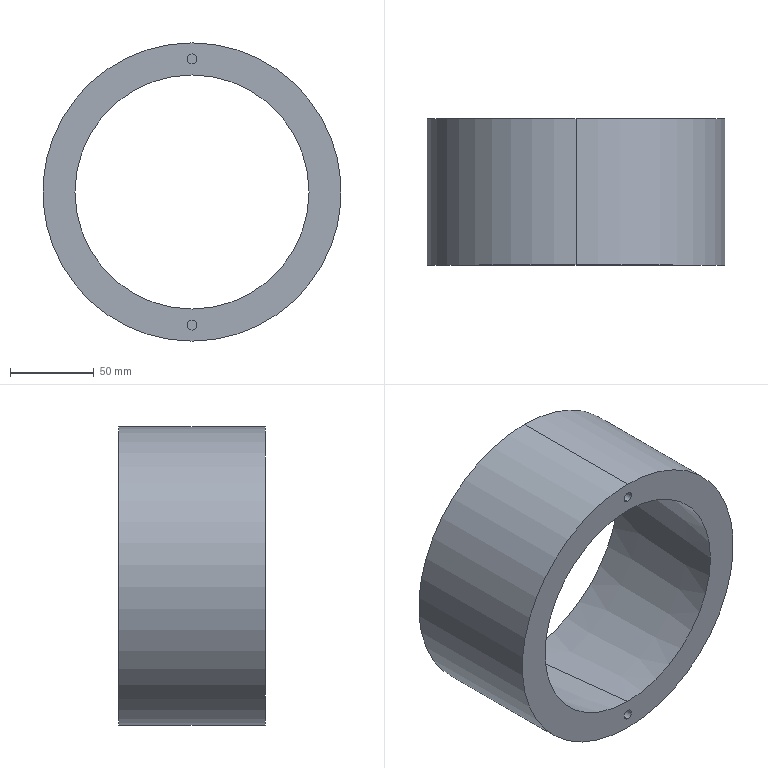Part | STEP file | waitao | 1 solid | 12 faces | box 178.3 x 87.518 x 178.3 mm | volume 654591 mm3 | cylinder 6 | plane 4 | cone 2 | commonest cylinder face diameters 6 x4 178.3 x2
STEP:
#1=CARTESIAN_POINT('',(0.,-167.046,82.551));
#2=VERTEX_POINT('',#1);
#3=CARTESIAN_POINT('',(0.,-167.046,76.551));
#4=VERTEX_POINT('',#3);
#5=CARTESIAN_POINT('',(0.,-167.046,79.551));
#6=DIRECTION('',(0.,-1.,0.));
#7=DIRECTION('',(0.,0.,-1.));
#8=AXIS2_PLACEMENT_3D('',#5,#6,#7);
#9=CIRCLE('',#8,3.);
#10=EDGE_CURVE('',#2,#4,#9,.T.);
#11=ORIENTED_EDGE('',*,*,#10,.F.);
#12=CARTESIAN_POINT('',(0.,-177.046,82.551));
#13=VERTEX_POINT('',#12);
#14=CARTESIAN_POINT('',(0.,-167.046,82.551));
#15=DIRECTION('',(0.,-1.,0.));
#16=VECTOR('',#15,1000.);
#17=LINE('',#14,#16);
#18=EDGE_CURVE('',#2,#13,#17,.T.);
#19=ORIENTED_EDGE('',*,*,#18,.T.);
#20=CARTESIAN_POINT('',(0.,-177.046,76.551));
#21=VERTEX_POINT('',#20);
#22=CARTESIAN_POINT('',(0.,-177.046,79.551));
#23=DIRECTION('',(0.,-1.,0.));
#24=DIRECTION('',(0.,0.,-1.));
#25=AXIS2_PLACEMENT_3D('',#22,#23,#24);
#26=CIRCLE('',#25,3.);
#27=EDGE_CURVE('',#13,#21,#26,.T.);
#28=ORIENTED_EDGE('',*,*,#27,.T.);
#29=CARTESIAN_POINT('',(0.,-167.046,76.551));
#30=DIRECTION('',(0.,-1.,0.));
#31=VECTOR('',#30,1000.);
#32=LINE('',#29,#31);
#33=EDGE_CURVE('',#4,#21,#32,.T.);
#34=ORIENTED_EDGE('',*,*,#33,.F.);
#35=EDGE_LOOP('',(#11,#19,#28,#34));
#36=FACE_OUTER_BOUND('',#35,.T.);
#37=CARTESIAN_POINT('',(0.,-167.046,79.551));
#38=DIRECTION('',(0.,-1.,0.));
#39=DIRECTION('',(0.,0.,-1.));
#40=AXIS2_PLACEMENT_3D('',#37,#38,#39);
#41=CYLINDRICAL_SURFACE('',#40,3.);
#42=ADVANCED_FACE('',(#36),#41,.F.);
#43=CARTESIAN_POINT('',(0.,-167.046,-76.551));
#44=VERTEX_POINT('',#43);
#45=CARTESIAN_POINT('',(0.,-167.046,-82.551));
#46=VERTEX_POINT('',#45);
#47=CARTESIAN_POINT('',(0.,-167.046,-79.551));
#48=DIRECTION('',(0.,-1.,0.));
#49=DIRECTION('',(0.,0.,-1.));
#50=AXIS2_PLACEMENT_3D('',#47,#48,#49);
#51=CIRCLE('',#50,3.);
#52=EDGE_CURVE('',#44,#46,#51,.T.);
#53=ORIENTED_EDGE('',*,*,#52,.F.);
#54=CARTESIAN_POINT('',(0.,-177.046,-76.551));
#55=VERTEX_POINT('',#54);
#56=CARTESIAN_POINT('',(0.,-167.046,-76.551));
#57=DIRECTION('',(0.,-1.,0.));
#58=VECTOR('',#57,1000.);
#59=LINE('',#56,#58);
#60=EDGE_CURVE('',#44,#55,#59,.T.);
#61=ORIENTED_EDGE('',*,*,#60,.T.);
#62=CARTESIAN_POINT('',(0.,-177.046,-82.551));
#63=VERTEX_POINT('',#62);
#64=CARTESIAN_POINT('',(0.,-177.046,-79.551));
#65=DIRECTION('',(0.,-1.,0.));
#66=DIRECTION('',(0.,0.,-1.));
#67=AXIS2_PLACEMENT_3D('',#64,#65,#66);
#68=CIRCLE('',#67,3.);
#69=EDGE_CURVE('',#55,#63,#68,.T.);
#70=ORIENTED_EDGE('',*,*,#69,.T.);
#71=CARTESIAN_POINT('',(0.,-167.046,-82.551));
#72=DIRECTION('',(0.,-1.,0.));
#73=VECTOR('',#72,1000.);
#74=LINE('',#71,#73);
#75=EDGE_CURVE('',#46,#63,#74,.T.);
#76=ORIENTED_EDGE('',*,*,#75,.F.);
#77=EDGE_LOOP('',(#53,#61,#70,#76));
#78=FACE_OUTER_BOUND('',#77,.T.);
#79=CARTESIAN_POINT('',(0.,-167.046,-79.551));
#80=DIRECTION('',(0.,-1.,0.));
#81=DIRECTION('',(0.,0.,-1.));
#82=AXIS2_PLACEMENT_3D('',#79,#80,#81);
#83=CYLINDRICAL_SURFACE('',#82,3.);
#84=ADVANCED_FACE('',(#78),#83,.F.);
#85=CARTESIAN_POINT('',(0.,-177.046,-69.951));
#86=VERTEX_POINT('',#85);
#87=CARTESIAN_POINT('',(0.,-177.046,69.951));
#88=VERTEX_POINT('',#87);
#89=CARTESIAN_POINT('',(0.,-177.046,0.));
#90=DIRECTION('',(0.,1.,0.));
#91=DIRECTION('',(0.,0.,1.));
#92=AXIS2_PLACEMENT_3D('',#89,#90,#91);
#93=CIRCLE('',#92,69.951);
#94=EDGE_CURVE('',#86,#88,#93,.T.);
#95=ORIENTED_EDGE('',*,*,#94,.F.);
#96=CARTESIAN_POINT('',(0.,-89.528,-79.15));
#97=VERTEX_POINT('',#96);
#98=CARTESIAN_POINT('',(0.,-89.528,-79.15));
#99=DIRECTION('',(0.,0.9945,-0.1045));
#100=VECTOR('',#99,1000.);
#101=LINE('',#98,#100);
#102=EDGE_CURVE('',#86,#97,#101,.T.);
#103=ORIENTED_EDGE('',*,*,#102,.T.);
#104=CARTESIAN_POINT('',(0.,-89.528,79.15));
#105=VERTEX_POINT('',#104);
#106=CARTESIAN_POINT('',(0.,-89.528,0.));
#107=DIRECTION('',(0.,1.,0.));
#108=DIRECTION('',(0.,0.,1.));
#109=AXIS2_PLACEMENT_3D('',#106,#107,#108);
#110=CIRCLE('',#109,79.15);
#111=EDGE_CURVE('',#97,#105,#110,.T.);
#112=ORIENTED_EDGE('',*,*,#111,.T.);
#113=CARTESIAN_POINT('',(0.,-89.528,79.15));
#114=DIRECTION('',(0.,0.9945,0.1045));
#115=VECTOR('',#114,1000.);
#116=LINE('',#113,#115);
#117=EDGE_CURVE('',#88,#105,#116,.T.);
#118=ORIENTED_EDGE('',*,*,#117,.F.);
#119=EDGE_LOOP('',(#95,#103,#112,#118));
#120=FACE_OUTER_BOUND('',#119,.T.);
#121=CARTESIAN_POINT('',(0.,-89.528,0.));
#122=DIRECTION('',(0.,1.,0.));
#123=DIRECTION('',(0.,0.,1.));
#124=AXIS2_PLACEMENT_3D('',#121,#122,#123);
#125=CONICAL_SURFACE('',#124,79.15,0.1047);
#126=ADVANCED_FACE('',(#120),#125,.F.);
#127=CARTESIAN_POINT('',(0.,-177.046,89.15));
#128=VERTEX_POINT('',#127);
#129=CARTESIAN_POINT('',(0.,-177.046,-89.15));
#130=VERTEX_POINT('',#129);
#131=CARTESIAN_POINT('',(0.,-177.046,0.));
#132=DIRECTION('',(0.,1.,0.));
#133=DIRECTION('',(0.,0.,1.));
#134=AXIS2_PLACEMENT_3D('',#131,#132,#133);
#135=CIRCLE('',#134,89.15);
#136=EDGE_CURVE('',#128,#130,#135,.T.);
#137=ORIENTED_EDGE('',*,*,#136,.T.);
#138=CARTESIAN_POINT('',(0.,-89.528,-89.15));
#139=VERTEX_POINT('',#138);
#140=CARTESIAN_POINT('',(0.,0.,-89.15));
#141=DIRECTION('',(0.,1.,0.));
#142=VECTOR('',#141,1000.);
#143=LINE('',#140,#142);
#144=EDGE_CURVE('',#130,#139,#143,.T.);
#145=ORIENTED_EDGE('',*,*,#144,.T.);
#146=CARTESIAN_POINT('',(0.,-89.528,89.15));
#147=VERTEX_POINT('',#146);
#148=CARTESIAN_POINT('',(0.,-89.528,0.));
#149=DIRECTION('',(0.,1.,0.));
#150=DIRECTION('',(0.,0.,1.));
#151=AXIS2_PLACEMENT_3D('',#148,#149,#150);
#152=CIRCLE('',#151,89.15);
#153=EDGE_CURVE('',#147,#139,#152,.T.);
#154=ORIENTED_EDGE('',*,*,#153,.F.);
#155=CARTESIAN_POINT('',(0.,0.,89.15));
#156=DIRECTION('',(0.,1.,0.));
#157=VECTOR('',#156,1000.);
#158=LINE('',#155,#157);
#159=EDGE_CURVE('',#128,#147,#158,.T.);
#160=ORIENTED_EDGE('',*,*,#159,.F.);
#161=EDGE_LOOP('',(#137,#145,#154,#160));
#162=FACE_OUTER_BOUND('',#161,.T.);
#163=CARTESIAN_POINT('',(0.,0.,0.));
#164=DIRECTION('',(0.,1.,0.));
#165=DIRECTION('',(0.,0.,1.));
#166=AXIS2_PLACEMENT_3D('',#163,#164,#165);
#167=CYLINDRICAL_SURFACE('',#166,89.15);
#168=ADVANCED_FACE('',(#162),#167,.T.);
#169=CARTESIAN_POINT('',(0.,-89.528,0.));
#170=DIRECTION('',(0.,1.,0.));
#171=DIRECTION('',(0.,0.,1.));
#172=AXIS2_PLACEMENT_3D('',#169,#170,#171);
#173=CIRCLE('',#172,79.15);
#174=EDGE_CURVE('',#105,#97,#173,.T.);
#175=ORIENTED_EDGE('',*,*,#174,.F.);
#176=ORIENTED_EDGE('',*,*,#111,.F.);
#177=EDGE_LOOP('',(#175,#176));
#178=FACE_BOUND('',#177,.T.);
#179=ORIENTED_EDGE('',*,*,#153,.T.);
#180=CARTESIAN_POINT('',(0.,-89.528,0.));
#181=DIRECTION('',(0.,1.,0.));
#182=DIRECTION('',(0.,0.,1.));
#183=AXIS2_PLACEMENT_3D('',#180,#181,#182);
#184=CIRCLE('',#183,89.15);
#185=EDGE_CURVE('',#139,#147,#184,.T.);
#186=ORIENTED_EDGE('',*,*,#185,.T.);
#187=EDGE_LOOP('',(#179,#186));
#188=FACE_OUTER_BOUND('',#187,.T.);
#189=CARTESIAN_POINT('',(79.15,-89.528,0.));
#190=DIRECTION('',(0.,-1.,0.));
#191=DIRECTION('',(0.,0.,-1.));
#192=AXIS2_PLACEMENT_3D('',#189,#190,#191);
#193=PLANE('',#192);
#194=ADVANCED_FACE('',(#178,#188),#193,.F.);
#195=ORIENTED_EDGE('',*,*,#144,.F.);
#196=CARTESIAN_POINT('',(0.,-177.046,0.));
#197=DIRECTION('',(0.,1.,0.));
#198=DIRECTION('',(0.,0.,1.));
#199=AXIS2_PLACEMENT_3D('',#196,#197,#198);
#200=CIRCLE('',#199,89.15);
#201=EDGE_CURVE('',#130,#128,#200,.T.);
#202=ORIENTED_EDGE('',*,*,#201,.T.);
#203=ORIENTED_EDGE('',*,*,#159,.T.);
#204=ORIENTED_EDGE('',*,*,#185,.F.);
#205=EDGE_LOOP('',(#195,#202,#203,#204));
#206=FACE_OUTER_BOUND('',#205,.T.);
#207=CARTESIAN_POINT('',(0.,0.,0.));
#208=DIRECTION('',(0.,1.,0.));
#209=DIRECTION('',(0.,0.,1.));
#210=AXIS2_PLACEMENT_3D('',#207,#208,#209);
#211=CYLINDRICAL_SURFACE('',#210,89.15);
#212=ADVANCED_FACE('',(#206),#211,.T.);
#213=CARTESIAN_POINT('',(0.,-177.046,79.551));
#214=DIRECTION('',(0.,-1.,0.));
#215=DIRECTION('',(0.,0.,-1.));
#216=AXIS2_PLACEMENT_3D('',#213,#214,#215);
#217=CIRCLE('',#216,3.);
#218=EDGE_CURVE('',#21,#13,#217,.T.);
#219=ORIENTED_EDGE('',*,*,#218,.F.);
#220=ORIENTED_EDGE('',*,*,#27,.F.);
#221=EDGE_LOOP('',(#219,#220));
#222=FACE_BOUND('',#221,.T.);
#223=CARTESIAN_POINT('',(0.,-177.046,-79.551));
#224=DIRECTION('',(0.,-1.,0.));
#225=DIRECTION('',(0.,0.,-1.));
#226=AXIS2_PLACEMENT_3D('',#223,#224,#225);
#227=CIRCLE('',#226,3.);
#228=EDGE_CURVE('',#63,#55,#227,.T.);
#229=ORIENTED_EDGE('',*,*,#228,.F.);
#230=ORIENTED_EDGE('',*,*,#69,.F.);
#231=EDGE_LOOP('',(#229,#230));
#232=FACE_BOUND('',#231,.T.);
#233=ORIENTED_EDGE('',*,*,#136,.F.);
#234=ORIENTED_EDGE('',*,*,#201,.F.);
#235=EDGE_LOOP('',(#233,#234));
#236=FACE_OUTER_BOUND('',#235,.T.);
#237=CARTESIAN_POINT('',(0.,-177.046,0.));
#238=DIRECTION('',(0.,1.,0.));
#239=DIRECTION('',(0.,0.,1.));
#240=AXIS2_PLACEMENT_3D('',#237,#238,#239);
#241=CIRCLE('',#240,69.951);
#242=EDGE_CURVE('',#88,#86,#241,.T.);
#243=ORIENTED_EDGE('',*,*,#242,.T.);
#244=ORIENTED_EDGE('',*,*,#94,.T.);
#245=EDGE_LOOP('',(#243,#244));
#246=FACE_BOUND('',#245,.T.);
#247=CARTESIAN_POINT('',(89.15,-177.046,0.));
#248=DIRECTION('',(0.,1.,0.));
#249=DIRECTION('',(0.,0.,1.));
#250=AXIS2_PLACEMENT_3D('',#247,#248,#249);
#251=PLANE('',#250);
#252=ADVANCED_FACE('',(#222,#232,#236,#246),#251,.F.);
#253=ORIENTED_EDGE('',*,*,#102,.F.);
#254=ORIENTED_EDGE('',*,*,#242,.F.);
#255=ORIENTED_EDGE('',*,*,#117,.T.);
#256=ORIENTED_EDGE('',*,*,#174,.T.);
#257=EDGE_LOOP('',(#253,#254,#255,#256));
#258=FACE_OUTER_BOUND('',#257,.T.);
#259=CARTESIAN_POINT('',(0.,-89.528,0.));
#260=DIRECTION('',(0.,1.,0.));
#261=DIRECTION('',(0.,0.,1.));
#262=AXIS2_PLACEMENT_3D('',#259,#260,#261);
#263=CONICAL_SURFACE('',#262,79.15,0.1047);
#264=ADVANCED_FACE('',(#258),#263,.F.);
#265=ORIENTED_EDGE('',*,*,#60,.F.);
#266=CARTESIAN_POINT('',(0.,-167.046,-79.551));
#267=DIRECTION('',(0.,-1.,0.));
#268=DIRECTION('',(0.,0.,-1.));
#269=AXIS2_PLACEMENT_3D('',#266,#267,#268);
#270=CIRCLE('',#269,3.);
#271=EDGE_CURVE('',#46,#44,#270,.T.);
#272=ORIENTED_EDGE('',*,*,#271,.F.);
#273=ORIENTED_EDGE('',*,*,#75,.T.);
#274=ORIENTED_EDGE('',*,*,#228,.T.);
#275=EDGE_LOOP('',(#265,#272,#273,#274));
#276=FACE_OUTER_BOUND('',#275,.T.);
#277=CARTESIAN_POINT('',(0.,-167.046,-79.551));
#278=DIRECTION('',(0.,-1.,0.));
#279=DIRECTION('',(0.,0.,-1.));
#280=AXIS2_PLACEMENT_3D('',#277,#278,#279);
#281=CYLINDRICAL_SURFACE('',#280,3.);
#282=ADVANCED_FACE('',(#276),#281,.F.);
#283=ORIENTED_EDGE('',*,*,#271,.T.);
#284=ORIENTED_EDGE('',*,*,#52,.T.);
#285=EDGE_LOOP('',(#283,#284));
#286=FACE_OUTER_BOUND('',#285,.T.);
#287=CARTESIAN_POINT('',(0.,-167.046,-79.551));
#288=DIRECTION('',(0.,-1.,0.));
#289=DIRECTION('',(0.,0.,-1.));
#290=AXIS2_PLACEMENT_3D('',#287,#288,#289);
#291=PLANE('',#290);
#292=ADVANCED_FACE('',(#286),#291,.T.);
#293=ORIENTED_EDGE('',*,*,#18,.F.);
#294=CARTESIAN_POINT('',(0.,-167.046,79.551));
#295=DIRECTION('',(0.,-1.,0.));
#296=DIRECTION('',(0.,0.,-1.));
#297=AXIS2_PLACEMENT_3D('',#294,#295,#296);
#298=CIRCLE('',#297,3.);
#299=EDGE_CURVE('',#4,#2,#298,.T.);
#300=ORIENTED_EDGE('',*,*,#299,.F.);
#301=ORIENTED_EDGE('',*,*,#33,.T.);
#302=ORIENTED_EDGE('',*,*,#218,.T.);
#303=EDGE_LOOP('',(#293,#300,#301,#302));
#304=FACE_OUTER_BOUND('',#303,.T.);
#305=CARTESIAN_POINT('',(0.,-167.046,79.551));
#306=DIRECTION('',(0.,-1.,0.));
#307=DIRECTION('',(0.,0.,-1.));
#308=AXIS2_PLACEMENT_3D('',#305,#306,#307);
#309=CYLINDRICAL_SURFACE('',#308,3.);
#310=ADVANCED_FACE('',(#304),#309,.F.);
#311=ORIENTED_EDGE('',*,*,#299,.T.);
#312=ORIENTED_EDGE('',*,*,#10,.T.);
#313=EDGE_LOOP('',(#311,#312));
#314=FACE_OUTER_BOUND('',#313,.T.);
#315=CARTESIAN_POINT('',(0.,-167.046,79.551));
#316=DIRECTION('',(0.,-1.,0.));
#317=DIRECTION('',(0.,0.,-1.));
#318=AXIS2_PLACEMENT_3D('',#315,#316,#317);
#319=PLANE('',#318);
#320=ADVANCED_FACE('',(#314),#319,.T.);
#321=CLOSED_SHELL('',(#42,#84,#126,#168,#194,#212,#252,#264,#282,#292,#310,#320));
#322=MANIFOLD_SOLID_BREP('',#321);
#323=CARTESIAN_POINT('',(0.,0.,0.));
#324=DIRECTION('',(0.,0.,1.));
#325=DIRECTION('',(1.,0.,0.));
#326=AXIS2_PLACEMENT_3D('',#323,#324,#325);
#327=(LENGTH_UNIT()NAMED_UNIT(*)SI_UNIT(.MILLI.,.METRE.));
#328=UNCERTAINTY_MEASURE_WITH_UNIT(LENGTH_MEASURE(0.00001),#327,'','');
#329=(NAMED_UNIT(*)PLANE_ANGLE_UNIT()SI_UNIT($,.RADIAN.));
#330=(NAMED_UNIT(*)SI_UNIT($,.STERADIAN.)SOLID_ANGLE_UNIT());
#331=(GEOMETRIC_REPRESENTATION_CONTEXT(3)GLOBAL_UNCERTAINTY_ASSIGNED_CONTEXT((#328))GLOBAL_UNIT_ASSIGNED_CONTEXT((#327,#329,#330))REPRESENTATION_CONTEXT('',''));
#332=ADVANCED_BREP_SHAPE_REPRESENTATION('',(#322,#326),#331);